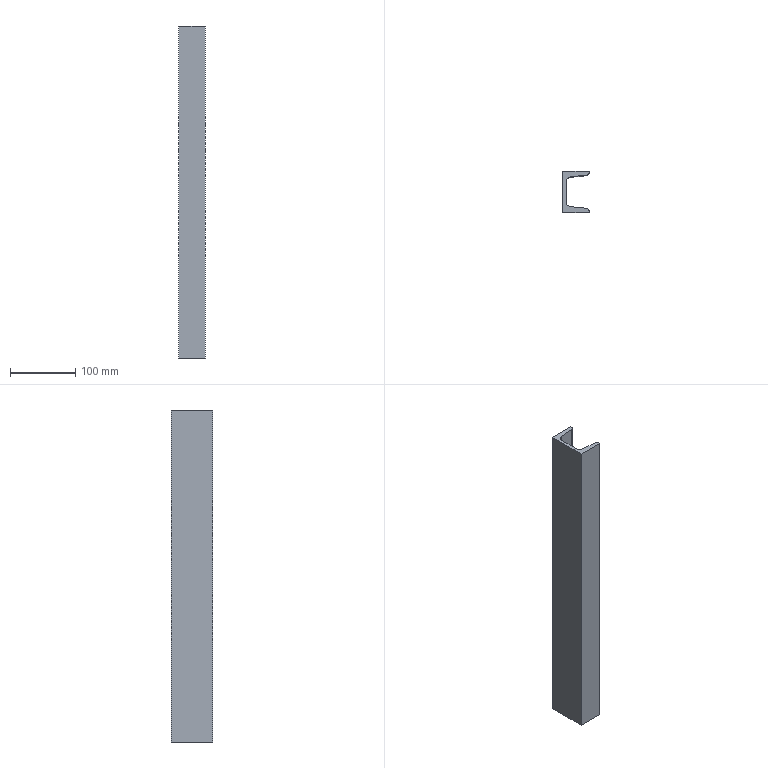Part | STEP file | 750038230 | 1 solid | 14 faces | box 40 x 63 x 510 mm | volume 430729 mm3 | plane 10 | cylinder 4 | commonest cylinder face diameters 7.6 x2 15 x2
STEP:
#1=CARTESIAN_POINT('',(0.,0.,255.));
#2=VERTEX_POINT('',#1);
#3=CARTESIAN_POINT('',(0.,0.,-255.));
#4=VERTEX_POINT('',#3);
#5=CARTESIAN_POINT('',(0.,0.,255.));
#6=DIRECTION('',(0.,0.,-1.));
#7=VECTOR('',#6,1000.);
#8=LINE('',#5,#7);
#9=EDGE_CURVE('',#2,#4,#8,.T.);
#10=ORIENTED_EDGE('',*,*,#9,.F.);
#11=CARTESIAN_POINT('',(0.,63.,255.));
#12=VERTEX_POINT('',#11);
#13=CARTESIAN_POINT('',(0.,63.,255.));
#14=DIRECTION('',(0.,-1.,0.));
#15=VECTOR('',#14,1000.);
#16=LINE('',#13,#15);
#17=EDGE_CURVE('',#12,#2,#16,.T.);
#18=ORIENTED_EDGE('',*,*,#17,.F.);
#19=CARTESIAN_POINT('',(0.,63.,-255.));
#20=VERTEX_POINT('',#19);
#21=CARTESIAN_POINT('',(0.,63.,255.));
#22=DIRECTION('',(0.,0.,1.));
#23=VECTOR('',#22,1000.);
#24=LINE('',#21,#23);
#25=EDGE_CURVE('',#20,#12,#24,.T.);
#26=ORIENTED_EDGE('',*,*,#25,.F.);
#27=CARTESIAN_POINT('',(0.,63.,-255.));
#28=DIRECTION('',(0.,1.,0.));
#29=VECTOR('',#28,1000.);
#30=LINE('',#27,#29);
#31=EDGE_CURVE('',#4,#20,#30,.T.);
#32=ORIENTED_EDGE('',*,*,#31,.F.);
#33=EDGE_LOOP('',(#10,#18,#26,#32));
#34=FACE_OUTER_BOUND('',#33,.T.);
#35=CARTESIAN_POINT('',(0.,63.,255.));
#36=DIRECTION('',(1.,0.,0.));
#37=DIRECTION('',(0.,0.,-1.));
#38=AXIS2_PLACEMENT_3D('',#35,#36,#37);
#39=PLANE('',#38);
#40=ADVANCED_FACE('',(#34),#39,.F.);
#41=CARTESIAN_POINT('',(40.,63.,-255.));
#42=VERTEX_POINT('',#41);
#43=CARTESIAN_POINT('',(36.2,63.,-255.));
#44=DIRECTION('',(-1.,0.,0.));
#45=VECTOR('',#44,1000.);
#46=LINE('',#43,#45);
#47=EDGE_CURVE('',#42,#20,#46,.T.);
#48=ORIENTED_EDGE('',*,*,#47,.F.);
#49=CARTESIAN_POINT('',(40.,60.699,-255.));
#50=VERTEX_POINT('',#49);
#51=CARTESIAN_POINT('',(40.,2.301,-255.));
#52=DIRECTION('',(0.,1.,0.));
#53=VECTOR('',#52,1000.);
#54=LINE('',#51,#53);
#55=EDGE_CURVE('',#50,#42,#54,.T.);
#56=ORIENTED_EDGE('',*,*,#55,.F.);
#57=CARTESIAN_POINT('',(36.578,56.918,-255.));
#58=VERTEX_POINT('',#57);
#59=CARTESIAN_POINT('',(36.2,60.699,-255.));
#60=DIRECTION('',(0.,0.,1.));
#61=DIRECTION('',(-1.,0.,0.));
#62=AXIS2_PLACEMENT_3D('',#59,#60,#61);
#63=CIRCLE('',#62,3.8);
#64=EDGE_CURVE('',#58,#50,#63,.T.);
#65=ORIENTED_EDGE('',*,*,#64,.F.);
#66=CARTESIAN_POINT('',(11.554,54.415,-255.));
#67=VERTEX_POINT('',#66);
#68=CARTESIAN_POINT('',(11.554,54.415,-255.));
#69=DIRECTION('',(0.995,0.0995,0.));
#70=VECTOR('',#69,1000.);
#71=LINE('',#68,#70);
#72=EDGE_CURVE('',#67,#58,#71,.T.);
#73=ORIENTED_EDGE('',*,*,#72,.F.);
#74=CARTESIAN_POINT('',(4.8,46.953,-255.));
#75=VERTEX_POINT('',#74);
#76=CARTESIAN_POINT('',(12.3,46.953,-255.));
#77=DIRECTION('',(0.,0.,-1.));
#78=DIRECTION('',(-1.,0.,0.));
#79=AXIS2_PLACEMENT_3D('',#76,#77,#78);
#80=CIRCLE('',#79,7.5);
#81=EDGE_CURVE('',#75,#67,#80,.T.);
#82=ORIENTED_EDGE('',*,*,#81,.F.);
#83=CARTESIAN_POINT('',(4.8,16.047,-255.));
#84=VERTEX_POINT('',#83);
#85=CARTESIAN_POINT('',(4.8,2.301,-255.));
#86=DIRECTION('',(0.,1.,0.));
#87=VECTOR('',#86,1000.);
#88=LINE('',#85,#87);
#89=EDGE_CURVE('',#84,#75,#88,.T.);
#90=ORIENTED_EDGE('',*,*,#89,.F.);
#91=CARTESIAN_POINT('',(11.554,8.585,-255.));
#92=VERTEX_POINT('',#91);
#93=CARTESIAN_POINT('',(12.3,16.047,-255.));
#94=DIRECTION('',(0.,0.,-1.));
#95=DIRECTION('',(-1.,0.,0.));
#96=AXIS2_PLACEMENT_3D('',#93,#94,#95);
#97=CIRCLE('',#96,7.5);
#98=EDGE_CURVE('',#92,#84,#97,.T.);
#99=ORIENTED_EDGE('',*,*,#98,.F.);
#100=CARTESIAN_POINT('',(36.578,6.082,-255.));
#101=VERTEX_POINT('',#100);
#102=CARTESIAN_POINT('',(36.578,6.082,-255.));
#103=DIRECTION('',(-0.995,0.0995,0.));
#104=VECTOR('',#103,1000.);
#105=LINE('',#102,#104);
#106=EDGE_CURVE('',#101,#92,#105,.T.);
#107=ORIENTED_EDGE('',*,*,#106,.F.);
#108=CARTESIAN_POINT('',(40.,2.301,-255.));
#109=VERTEX_POINT('',#108);
#110=CARTESIAN_POINT('',(36.2,2.301,-255.));
#111=DIRECTION('',(0.,0.,1.));
#112=DIRECTION('',(-1.,0.,0.));
#113=AXIS2_PLACEMENT_3D('',#110,#111,#112);
#114=CIRCLE('',#113,3.8);
#115=EDGE_CURVE('',#109,#101,#114,.T.);
#116=ORIENTED_EDGE('',*,*,#115,.F.);
#117=CARTESIAN_POINT('',(40.,0.,-255.));
#118=VERTEX_POINT('',#117);
#119=CARTESIAN_POINT('',(40.,2.301,-255.));
#120=DIRECTION('',(0.,1.,0.));
#121=VECTOR('',#120,1000.);
#122=LINE('',#119,#121);
#123=EDGE_CURVE('',#118,#109,#122,.T.);
#124=ORIENTED_EDGE('',*,*,#123,.F.);
#125=CARTESIAN_POINT('',(36.2,0.,-255.));
#126=DIRECTION('',(1.,0.,0.));
#127=VECTOR('',#126,1000.);
#128=LINE('',#125,#127);
#129=EDGE_CURVE('',#4,#118,#128,.T.);
#130=ORIENTED_EDGE('',*,*,#129,.F.);
#131=ORIENTED_EDGE('',*,*,#31,.T.);
#132=EDGE_LOOP('',(#48,#56,#65,#73,#82,#90,#99,#107,#116,#124,#130,#131));
#133=FACE_OUTER_BOUND('',#132,.T.);
#134=CARTESIAN_POINT('',(36.2,2.301,-255.));
#135=DIRECTION('',(0.,0.,1.));
#136=DIRECTION('',(1.,0.,0.));
#137=AXIS2_PLACEMENT_3D('',#134,#135,#136);
#138=PLANE('',#137);
#139=ADVANCED_FACE('',(#133),#138,.F.);
#140=CARTESIAN_POINT('',(40.,0.,255.));
#141=VERTEX_POINT('',#140);
#142=CARTESIAN_POINT('',(40.,0.,255.));
#143=DIRECTION('',(0.,0.,-1.));
#144=VECTOR('',#143,1000.);
#145=LINE('',#142,#144);
#146=EDGE_CURVE('',#141,#118,#145,.T.);
#147=ORIENTED_EDGE('',*,*,#146,.F.);
#148=CARTESIAN_POINT('',(0.,0.,255.));
#149=DIRECTION('',(1.,0.,0.));
#150=VECTOR('',#149,1000.);
#151=LINE('',#148,#150);
#152=EDGE_CURVE('',#2,#141,#151,.T.);
#153=ORIENTED_EDGE('',*,*,#152,.F.);
#154=ORIENTED_EDGE('',*,*,#9,.T.);
#155=ORIENTED_EDGE('',*,*,#129,.T.);
#156=EDGE_LOOP('',(#147,#153,#154,#155));
#157=FACE_OUTER_BOUND('',#156,.T.);
#158=CARTESIAN_POINT('',(0.,0.,255.));
#159=DIRECTION('',(0.,1.,0.));
#160=DIRECTION('',(0.,0.,1.));
#161=AXIS2_PLACEMENT_3D('',#158,#159,#160);
#162=PLANE('',#161);
#163=ADVANCED_FACE('',(#157),#162,.F.);
#164=CARTESIAN_POINT('',(40.,60.699,255.));
#165=VERTEX_POINT('',#164);
#166=CARTESIAN_POINT('',(40.,63.,255.));
#167=VERTEX_POINT('',#166);
#168=CARTESIAN_POINT('',(40.,2.301,255.));
#169=DIRECTION('',(0.,1.,0.));
#170=VECTOR('',#169,1000.);
#171=LINE('',#168,#170);
#172=EDGE_CURVE('',#165,#167,#171,.T.);
#173=ORIENTED_EDGE('',*,*,#172,.T.);
#174=CARTESIAN_POINT('',(36.2,63.,255.));
#175=DIRECTION('',(-1.,0.,0.));
#176=VECTOR('',#175,1000.);
#177=LINE('',#174,#176);
#178=EDGE_CURVE('',#167,#12,#177,.T.);
#179=ORIENTED_EDGE('',*,*,#178,.T.);
#180=ORIENTED_EDGE('',*,*,#17,.T.);
#181=ORIENTED_EDGE('',*,*,#152,.T.);
#182=CARTESIAN_POINT('',(40.,2.301,255.));
#183=VERTEX_POINT('',#182);
#184=CARTESIAN_POINT('',(40.,2.301,255.));
#185=DIRECTION('',(0.,1.,0.));
#186=VECTOR('',#185,1000.);
#187=LINE('',#184,#186);
#188=EDGE_CURVE('',#141,#183,#187,.T.);
#189=ORIENTED_EDGE('',*,*,#188,.T.);
#190=CARTESIAN_POINT('',(36.578,6.082,255.));
#191=VERTEX_POINT('',#190);
#192=CARTESIAN_POINT('',(36.2,2.301,255.));
#193=DIRECTION('',(0.,0.,1.));
#194=DIRECTION('',(-1.,0.,0.));
#195=AXIS2_PLACEMENT_3D('',#192,#193,#194);
#196=CIRCLE('',#195,3.8);
#197=EDGE_CURVE('',#183,#191,#196,.T.);
#198=ORIENTED_EDGE('',*,*,#197,.T.);
#199=CARTESIAN_POINT('',(11.554,8.585,255.));
#200=VERTEX_POINT('',#199);
#201=CARTESIAN_POINT('',(36.578,6.082,255.));
#202=DIRECTION('',(-0.995,0.0995,0.));
#203=VECTOR('',#202,1000.);
#204=LINE('',#201,#203);
#205=EDGE_CURVE('',#191,#200,#204,.T.);
#206=ORIENTED_EDGE('',*,*,#205,.T.);
#207=CARTESIAN_POINT('',(4.8,16.047,255.));
#208=VERTEX_POINT('',#207);
#209=CARTESIAN_POINT('',(12.3,16.047,255.));
#210=DIRECTION('',(0.,0.,-1.));
#211=DIRECTION('',(-1.,0.,0.));
#212=AXIS2_PLACEMENT_3D('',#209,#210,#211);
#213=CIRCLE('',#212,7.5);
#214=EDGE_CURVE('',#200,#208,#213,.T.);
#215=ORIENTED_EDGE('',*,*,#214,.T.);
#216=CARTESIAN_POINT('',(4.8,46.953,255.));
#217=VERTEX_POINT('',#216);
#218=CARTESIAN_POINT('',(4.8,2.301,255.));
#219=DIRECTION('',(0.,1.,0.));
#220=VECTOR('',#219,1000.);
#221=LINE('',#218,#220);
#222=EDGE_CURVE('',#208,#217,#221,.T.);
#223=ORIENTED_EDGE('',*,*,#222,.T.);
#224=CARTESIAN_POINT('',(11.554,54.415,255.));
#225=VERTEX_POINT('',#224);
#226=CARTESIAN_POINT('',(12.3,46.953,255.));
#227=DIRECTION('',(0.,0.,-1.));
#228=DIRECTION('',(-1.,0.,0.));
#229=AXIS2_PLACEMENT_3D('',#226,#227,#228);
#230=CIRCLE('',#229,7.5);
#231=EDGE_CURVE('',#217,#225,#230,.T.);
#232=ORIENTED_EDGE('',*,*,#231,.T.);
#233=CARTESIAN_POINT('',(36.578,56.918,255.));
#234=VERTEX_POINT('',#233);
#235=CARTESIAN_POINT('',(11.554,54.415,255.));
#236=DIRECTION('',(0.995,0.0995,0.));
#237=VECTOR('',#236,1000.);
#238=LINE('',#235,#237);
#239=EDGE_CURVE('',#225,#234,#238,.T.);
#240=ORIENTED_EDGE('',*,*,#239,.T.);
#241=CARTESIAN_POINT('',(36.2,60.699,255.));
#242=DIRECTION('',(0.,0.,1.));
#243=DIRECTION('',(-1.,0.,0.));
#244=AXIS2_PLACEMENT_3D('',#241,#242,#243);
#245=CIRCLE('',#244,3.8);
#246=EDGE_CURVE('',#234,#165,#245,.T.);
#247=ORIENTED_EDGE('',*,*,#246,.T.);
#248=EDGE_LOOP('',(#173,#179,#180,#181,#189,#198,#206,#215,#223,#232,#240,#247));
#249=FACE_OUTER_BOUND('',#248,.T.);
#250=CARTESIAN_POINT('',(36.2,2.301,255.));
#251=DIRECTION('',(0.,0.,1.));
#252=DIRECTION('',(1.,0.,0.));
#253=AXIS2_PLACEMENT_3D('',#250,#251,#252);
#254=PLANE('',#253);
#255=ADVANCED_FACE('',(#249),#254,.T.);
#256=ORIENTED_EDGE('',*,*,#25,.T.);
#257=ORIENTED_EDGE('',*,*,#178,.F.);
#258=CARTESIAN_POINT('',(40.,63.,255.));
#259=DIRECTION('',(0.,0.,1.));
#260=VECTOR('',#259,1000.);
#261=LINE('',#258,#260);
#262=EDGE_CURVE('',#42,#167,#261,.T.);
#263=ORIENTED_EDGE('',*,*,#262,.F.);
#264=ORIENTED_EDGE('',*,*,#47,.T.);
#265=EDGE_LOOP('',(#256,#257,#263,#264));
#266=FACE_OUTER_BOUND('',#265,.T.);
#267=CARTESIAN_POINT('',(40.,63.,255.));
#268=DIRECTION('',(0.,-1.,0.));
#269=DIRECTION('',(0.,0.,-1.));
#270=AXIS2_PLACEMENT_3D('',#267,#268,#269);
#271=PLANE('',#270);
#272=ADVANCED_FACE('',(#266),#271,.F.);
#273=ORIENTED_EDGE('',*,*,#262,.T.);
#274=ORIENTED_EDGE('',*,*,#172,.F.);
#275=CARTESIAN_POINT('',(40.,60.699,255.));
#276=DIRECTION('',(0.,0.,1.));
#277=VECTOR('',#276,1000.);
#278=LINE('',#275,#277);
#279=EDGE_CURVE('',#50,#165,#278,.T.);
#280=ORIENTED_EDGE('',*,*,#279,.F.);
#281=ORIENTED_EDGE('',*,*,#55,.T.);
#282=EDGE_LOOP('',(#273,#274,#280,#281));
#283=FACE_OUTER_BOUND('',#282,.T.);
#284=CARTESIAN_POINT('',(40.,60.699,255.));
#285=DIRECTION('',(-1.,0.,0.));
#286=DIRECTION('',(0.,-1.,0.));
#287=AXIS2_PLACEMENT_3D('',#284,#285,#286);
#288=PLANE('',#287);
#289=ADVANCED_FACE('',(#283),#288,.F.);
#290=ORIENTED_EDGE('',*,*,#246,.F.);
#291=CARTESIAN_POINT('',(36.578,56.918,255.));
#292=DIRECTION('',(0.,0.,-1.));
#293=VECTOR('',#292,1000.);
#294=LINE('',#291,#293);
#295=EDGE_CURVE('',#234,#58,#294,.T.);
#296=ORIENTED_EDGE('',*,*,#295,.T.);
#297=ORIENTED_EDGE('',*,*,#64,.T.);
#298=ORIENTED_EDGE('',*,*,#279,.T.);
#299=EDGE_LOOP('',(#290,#296,#297,#298));
#300=FACE_OUTER_BOUND('',#299,.T.);
#301=CARTESIAN_POINT('',(36.2,60.699,255.));
#302=DIRECTION('',(0.,0.,-1.));
#303=DIRECTION('',(-1.,0.,0.));
#304=AXIS2_PLACEMENT_3D('',#301,#302,#303);
#305=CYLINDRICAL_SURFACE('',#304,3.8);
#306=ADVANCED_FACE('',(#300),#305,.T.);
#307=ORIENTED_EDGE('',*,*,#295,.F.);
#308=ORIENTED_EDGE('',*,*,#239,.F.);
#309=CARTESIAN_POINT('',(11.554,54.415,255.));
#310=DIRECTION('',(0.,0.,1.));
#311=VECTOR('',#310,1000.);
#312=LINE('',#309,#311);
#313=EDGE_CURVE('',#67,#225,#312,.T.);
#314=ORIENTED_EDGE('',*,*,#313,.F.);
#315=ORIENTED_EDGE('',*,*,#72,.T.);
#316=EDGE_LOOP('',(#307,#308,#314,#315));
#317=FACE_OUTER_BOUND('',#316,.T.);
#318=CARTESIAN_POINT('',(11.554,54.415,255.));
#319=DIRECTION('',(-0.0995,0.995,0.));
#320=DIRECTION('',(-0.995,-0.0995,0.));
#321=AXIS2_PLACEMENT_3D('',#318,#319,#320);
#322=PLANE('',#321);
#323=ADVANCED_FACE('',(#317),#322,.F.);
#324=ORIENTED_EDGE('',*,*,#313,.T.);
#325=ORIENTED_EDGE('',*,*,#231,.F.);
#326=CARTESIAN_POINT('',(4.8,46.953,255.));
#327=DIRECTION('',(0.,0.,1.));
#328=VECTOR('',#327,1000.);
#329=LINE('',#326,#328);
#330=EDGE_CURVE('',#75,#217,#329,.T.);
#331=ORIENTED_EDGE('',*,*,#330,.F.);
#332=ORIENTED_EDGE('',*,*,#81,.T.);
#333=EDGE_LOOP('',(#324,#325,#331,#332));
#334=FACE_OUTER_BOUND('',#333,.T.);
#335=CARTESIAN_POINT('',(12.3,46.953,255.));
#336=DIRECTION('',(0.,0.,-1.));
#337=DIRECTION('',(-1.,0.,0.));
#338=AXIS2_PLACEMENT_3D('',#335,#336,#337);
#339=CYLINDRICAL_SURFACE('',#338,7.5);
#340=ADVANCED_FACE('',(#334),#339,.F.);
#341=ORIENTED_EDGE('',*,*,#330,.T.);
#342=ORIENTED_EDGE('',*,*,#222,.F.);
#343=CARTESIAN_POINT('',(4.8,16.047,255.));
#344=DIRECTION('',(0.,0.,1.));
#345=VECTOR('',#344,1000.);
#346=LINE('',#343,#345);
#347=EDGE_CURVE('',#84,#208,#346,.T.);
#348=ORIENTED_EDGE('',*,*,#347,.F.);
#349=ORIENTED_EDGE('',*,*,#89,.T.);
#350=EDGE_LOOP('',(#341,#342,#348,#349));
#351=FACE_OUTER_BOUND('',#350,.T.);
#352=CARTESIAN_POINT('',(4.8,16.047,255.));
#353=DIRECTION('',(-1.,0.,0.));
#354=DIRECTION('',(0.,-1.,0.));
#355=AXIS2_PLACEMENT_3D('',#352,#353,#354);
#356=PLANE('',#355);
#357=ADVANCED_FACE('',(#351),#356,.F.);
#358=ORIENTED_EDGE('',*,*,#347,.T.);
#359=ORIENTED_EDGE('',*,*,#214,.F.);
#360=CARTESIAN_POINT('',(11.554,8.585,255.));
#361=DIRECTION('',(0.,0.,1.));
#362=VECTOR('',#361,1000.);
#363=LINE('',#360,#362);
#364=EDGE_CURVE('',#92,#200,#363,.T.);
#365=ORIENTED_EDGE('',*,*,#364,.F.);
#366=ORIENTED_EDGE('',*,*,#98,.T.);
#367=EDGE_LOOP('',(#358,#359,#365,#366));
#368=FACE_OUTER_BOUND('',#367,.T.);
#369=CARTESIAN_POINT('',(12.3,16.047,255.));
#370=DIRECTION('',(0.,0.,-1.));
#371=DIRECTION('',(-1.,0.,0.));
#372=AXIS2_PLACEMENT_3D('',#369,#370,#371);
#373=CYLINDRICAL_SURFACE('',#372,7.5);
#374=ADVANCED_FACE('',(#368),#373,.F.);
#375=ORIENTED_EDGE('',*,*,#364,.T.);
#376=ORIENTED_EDGE('',*,*,#205,.F.);
#377=CARTESIAN_POINT('',(36.578,6.082,255.));
#378=DIRECTION('',(0.,0.,1.));
#379=VECTOR('',#378,1000.);
#380=LINE('',#377,#379);
#381=EDGE_CURVE('',#101,#191,#380,.T.);
#382=ORIENTED_EDGE('',*,*,#381,.F.);
#383=ORIENTED_EDGE('',*,*,#106,.T.);
#384=EDGE_LOOP('',(#375,#376,#382,#383));
#385=FACE_OUTER_BOUND('',#384,.T.);
#386=CARTESIAN_POINT('',(36.578,6.082,255.));
#387=DIRECTION('',(-0.0995,-0.995,0.));
#388=DIRECTION('',(0.995,-0.0995,0.));
#389=AXIS2_PLACEMENT_3D('',#386,#387,#388);
#390=PLANE('',#389);
#391=ADVANCED_FACE('',(#385),#390,.F.);
#392=ORIENTED_EDGE('',*,*,#197,.F.);
#393=CARTESIAN_POINT('',(40.,2.301,255.));
#394=DIRECTION('',(0.,0.,-1.));
#395=VECTOR('',#394,1000.);
#396=LINE('',#393,#395);
#397=EDGE_CURVE('',#183,#109,#396,.T.);
#398=ORIENTED_EDGE('',*,*,#397,.T.);
#399=ORIENTED_EDGE('',*,*,#115,.T.);
#400=ORIENTED_EDGE('',*,*,#381,.T.);
#401=EDGE_LOOP('',(#392,#398,#399,#400));
#402=FACE_OUTER_BOUND('',#401,.T.);
#403=CARTESIAN_POINT('',(36.2,2.301,255.));
#404=DIRECTION('',(0.,0.,-1.));
#405=DIRECTION('',(-1.,0.,0.));
#406=AXIS2_PLACEMENT_3D('',#403,#404,#405);
#407=CYLINDRICAL_SURFACE('',#406,3.8);
#408=ADVANCED_FACE('',(#402),#407,.T.);
#409=ORIENTED_EDGE('',*,*,#397,.F.);
#410=ORIENTED_EDGE('',*,*,#188,.F.);
#411=ORIENTED_EDGE('',*,*,#146,.T.);
#412=ORIENTED_EDGE('',*,*,#123,.T.);
#413=EDGE_LOOP('',(#409,#410,#411,#412));
#414=FACE_OUTER_BOUND('',#413,.T.);
#415=CARTESIAN_POINT('',(40.,0.,255.));
#416=DIRECTION('',(-1.,0.,0.));
#417=DIRECTION('',(0.,0.,1.));
#418=AXIS2_PLACEMENT_3D('',#415,#416,#417);
#419=PLANE('',#418);
#420=ADVANCED_FACE('',(#414),#419,.F.);
#421=CLOSED_SHELL('',(#40,#139,#163,#255,#272,#289,#306,#323,#340,#357,#374,#391,#408,#420));
#422=MANIFOLD_SOLID_BREP('',#421);
#423=CARTESIAN_POINT('',(0.,0.,0.));
#424=DIRECTION('',(0.,0.,1.));
#425=DIRECTION('',(1.,0.,0.));
#426=AXIS2_PLACEMENT_3D('',#423,#424,#425);
#427=(LENGTH_UNIT()NAMED_UNIT(*)SI_UNIT(.MILLI.,.METRE.));
#428=UNCERTAINTY_MEASURE_WITH_UNIT(LENGTH_MEASURE(0.00001),#427,'','');
#429=(NAMED_UNIT(*)PLANE_ANGLE_UNIT()SI_UNIT($,.RADIAN.));
#430=(NAMED_UNIT(*)SI_UNIT($,.STERADIAN.)SOLID_ANGLE_UNIT());
#431=(GEOMETRIC_REPRESENTATION_CONTEXT(3)GLOBAL_UNCERTAINTY_ASSIGNED_CONTEXT((#428))GLOBAL_UNIT_ASSIGNED_CONTEXT((#427,#429,#430))REPRESENTATION_CONTEXT('',''));
#432=ADVANCED_BREP_SHAPE_REPRESENTATION('',(#422,#426),#431);